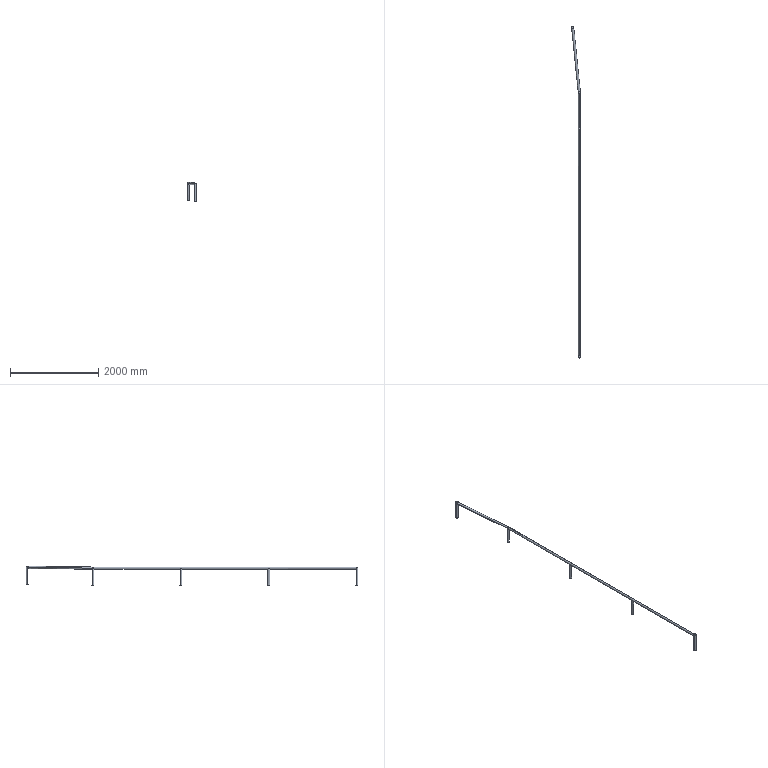Part | STEP file | Guide_default<machined> | 7 solids | 31 faces | box 201.365 x 7542 x 441.673 mm | volume 18501367 mm3 | cylinder 21 | plane 10 | commonest cylinder face diameters 50 x21